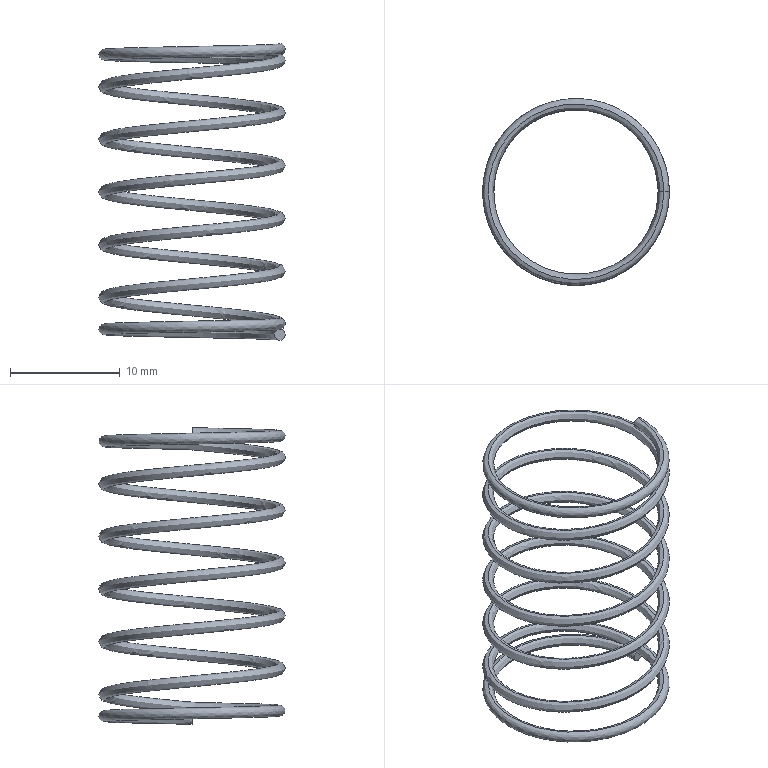Part | SolidWorks | features Helix 1, Sweep 1 | 1 solid | 4 faces | box 17 x 17 x 27.04 mm | volume 272.389 mm3 | spline 2 | plane 2